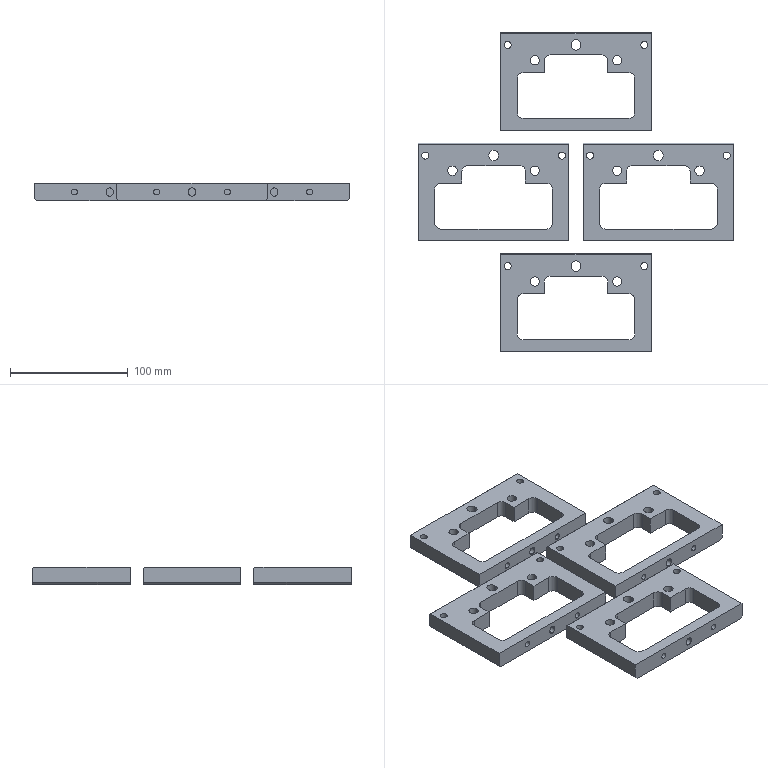CAM job | NX | 3+2 milling, drilling | part box 268 x 271 x 15 mm
Tools:
number,name,description,diameter,corner_radius,flute_length,length,flutes
7,D6A45,Milling Tool-5 Parameters,6.0,0.0,50.0,75.0,2
16,6.0ZT,Drilling Tool,6.0,0.0,35.0,50.0,2
4,D4,Milling Tool-5 Parameters,4.0,0.0,50.0,75.0,2
10,D10,Milling Tool-5 Parameters,10.0,0.0,50.0,75.0,2
11,D10JING,Milling Tool-5 Parameters,10.0,0.0,50.0,75.0,2
15,5.0ZT,Drilling Tool,5.0,0.0,35.0,50.0,2
Operations:
program,operation,operation_type,tool,method,geometry_group,spindle_rpm,surface_speed,feed_per_tooth,feed_cut,feed_plunge,cut_length_mm,path_length_mm,cut_time_min,machine_time_min
1,DRILLING,Operation,D6A45,METHOD,A,5000.0,94.0,0.025,250.0,0.0,80.0,1046.349,0.32,0.4166
1,DRILLING_COPY,Operation,6.0ZT,METHOD,A,2000.0,28.0,0.05,200.0,0.0,170.421,1123.174,0.8521,0.9474
1,DRILLING_COPY_COPY,Operation,6.0ZT,METHOD,A,2000.0,28.0,0.05,200.0,0.0,255.631,1210.661,1.278,1.374
1,PLANAR_MILL,PlanarMilling,D10,METHOD,A,9500.0,298.0,0.1579,3000.0,1000.0,143362.23,149082.391,50.335,50.907
1,ZLEVEL_PROFILE,ZLevelMilling,D10,METHOD,A,9500.0,298.0,0.1579,3000.0,1000.0,91021.375,91851.219,30.432,30.515
1,CAVITY_MILL_COPY_1,CavityMilling,D10JING,METHOD,A,9500.0,298.0,0.0632,1200.0,1000.0,1084.186,1825.323,0.9059,0.98
1,ZLEVEL_PROFILE_COPY_1,ZLevelMilling,D10JING,METHOD,A,9500.0,298.0,0.0632,1200.0,1000.0,1826.604,2607.408,1.523,1.601
1,HOLE_MILLING,CylinderMilling,D4,METHOD,A,9500.0,119.0,0.0868,1650.0,100.0,3846.13,5027.33,2.331,2.449
1,ZLEVEL_PROFILE_COPY,ZLevelMilling,D4,METHOD,A,9500.0,119.0,0.0632,1200.0,1000.0,4351.657,4993.793,3.648,3.712
1,PLANAR_MILL_1,PlanarMilling,D6A45,METHOD,A,9500.0,179.0,0.0658,1250.0,100.0,3287.599,6050.759,2.63,2.906
1,TOOLCOMP,CylinderMilling,D4,METHOD,A,9500.0,119.0,0.0632,1200.0,100.0,917.029,2098.23,0.7642,0.8823
1,TOOLCOMP4,ZLevelMilling,D4,METHOD,A,9500.0,119.0,0.0632,1200.0,1000.0,630.444,1281.927,0.5266,0.5918
2,DRILLING_COPY_1,Operation,D6A45,METHOD,B,5000.0,94.0,0.025,250.0,0.0,12.0,150.308,0.048,0.0618
2,DRILLING_COPY_COPY_1,Operation,5.0ZT,METHOD,B,2000.0,28.0,0.05,200.0,0.0,43.004,212.316,0.215,0.232
2,ZLEVEL_PROFILE_COPY_COPY,ZLevelMilling,D4,METHOD,B,9500.0,119.0,0.0632,1200.0,1000.0,344.757,409.757,0.2927,0.2992
2,PLANAR_MILL_1_COPY,PlanarMilling,D6A45,METHOD,B,9500.0,179.0,0.0658,1250.0,100.0,49.175,288.993,0.0393,0.0633
2,TOOLCOMP4_COPY,ZLevelMilling,D4,METHOD,B,9500.0,119.0,0.0632,1200.0,1000.0,57.75,125.083,0.0484,0.0551